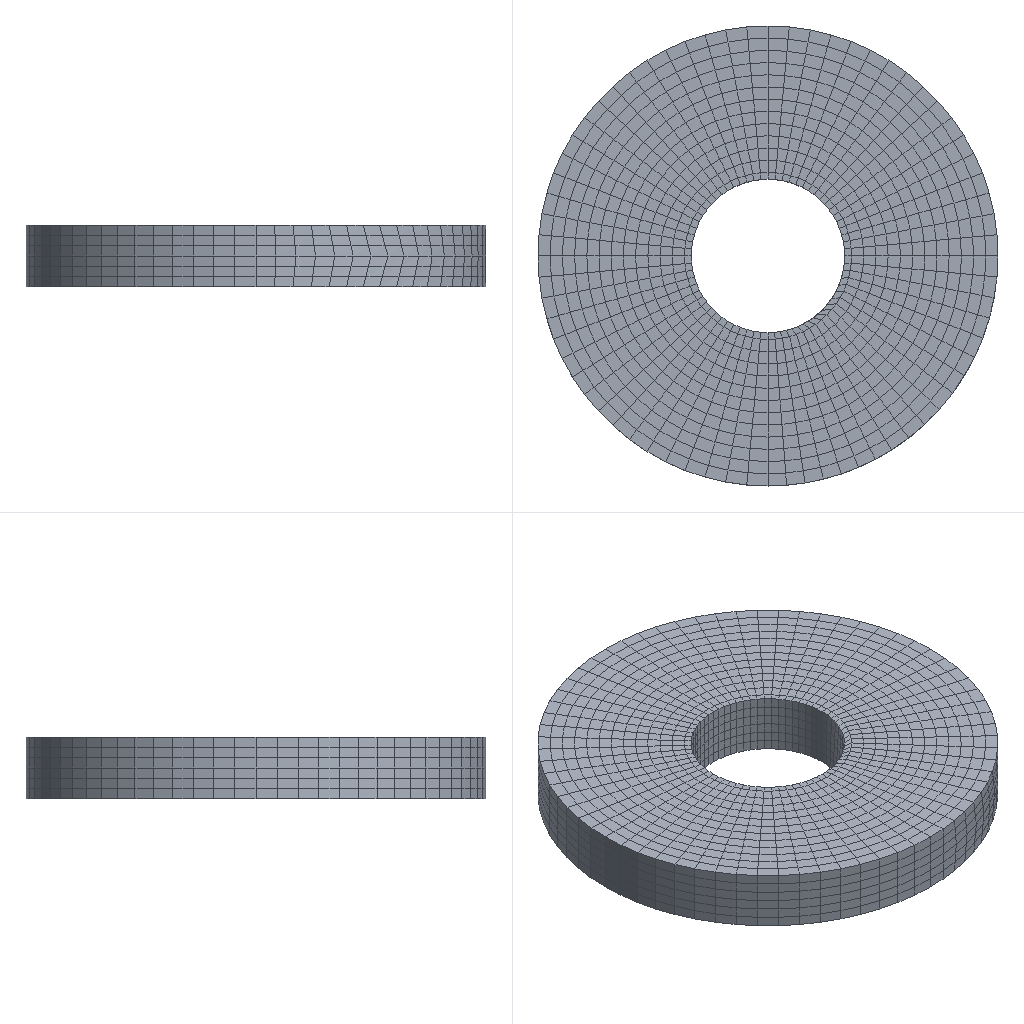Simulation study | abaqus
Set-up summary:
category,name,step,type,value,unit,region
solver,abaqus
solver,version,,,Abaqus/Standard 2020
units,not stated in the deck,,not stated
analysis,deck,,transient,transient
load_step,Step-1,Step-1,transient
load_step,requested,,,1
mesh,nodes,,,8353
mesh,elements,,,6735
element_type,C3D8,,solid,5382
element_type,R3D3,,rigid,14
element_type,R3D4,,rigid,1270
element_type,COH3D8,,cohesive,69
load,load commands in deck,,count,1
bc,support commands in deck,,count,1
material,MATERIAL-1,,in results
material,MATERIAL-1-COPY,,in results
check,setup vs results,,match,"per instance, exact: element labels, types and connectivity; labels of the nodes the elements use; coordinates of those nodes at SINGLE_PRECISION in 2 of 2 instance(s)"
Abaqus input file, long lists of numbers shortened:
*Heading
** Job name: Job-2 Model name: Model-1-Copy
** Generated by: Abaqus/CAE 2020
*Preprint, echo=NO, model=NO, history=NO, contact=NO
**
** PARTS
**
*Part, name=Part-1
*Node
      1,   1.118,  -2.236,           4.
      2,   1.118,  -2.236,           0.
** (1277 more lines like these left out)
*Element, type=R3D4
  1,   1,   3, 105, 156
  2,   3,   4, 106, 105
** (1268 more lines like these left out)
*Element, type=R3D3
677,  963,  757,  736
678,  987,  863,  818
** (12 more lines like these left out)
*Node
   1280,           0., -1.5308085e-16,           4.
*Nset, nset=Part-1-RefPt_, internal
1280,
*Elset, elset=Part-1, generate
    1,  1284,     1
*End Part
**
*Part, name=Part-2
*Node
      1,   2.723,           0.,           1.
      2,          2.5,           0.,           1.
** (7071 more lines like these left out)
*Element, type=C3D8
 1,  108,  111,  834,  802,    1, 6763, 6764,   72
 2,  802,  834,  835,  803,   72, 6764, 6765,   71
** (5380 more lines like these left out)
*Element, type=COH3D8
5383,   72,   41,    2,    1,   72, 6764, 6763,    1
5384,   71,   42,   41,   72,   71, 6765, 6764,   72
** (67 more lines like these left out)
*Nset, nset=Set-3, generate
    1,  6831,     1
*Elset, elset=Set-3, generate
    1,  5382,     1
*Nset, nset=Set-11
    1,    4,    7,    8,    9,   13,   14,   17,   18,   19,   20,   21,   22,   23,   24,   25
   26,   27,   30,   31,   34,   36,   37,   38,   39,   40,   57,   58,   59,   60,   61,   62
** (391 more lines like these left out)
*Elset, elset=Set-11
  157,  158,  159,  160,  161,  162,  163,  164,  165,  166,  167,  168,  169,  170,  171,  172
  173,  174,  175,  176,  177,  178,  179,  180,  181,  182,  183,  184,  185,  186,  187,  188
** (309 more lines like these left out)
*Nset, nset=Set-12, generate
    1,  6831,     1
*Elset, elset=Set-12, generate
    1,  5382,     1
*Elset, elset=CohesiveSeam-1-Elements, generate
 5383,  5451,     1
*Nset, nset=CohesiveSeam-1-TopNodes
    1,    4,    9,   14,   57,   58,   59,   60,   61,   62,   63,   64,   65,   66,   67,   68
   69,   70,   71,   72,  130,  131,  132,  133,  134,  135,  136,  137,  138,  139,  140,  141
** (7 more lines like these left out)
*Nset, nset=CohesiveSeam-1-BottomNodes
   1,   2,   3,   4,   9,  10,  14,  15,  41,  42,  43,  44,  45,  46,  47,  48
  49,  50,  51,  52,  53,  54,  55,  56,  57,  58,  59,  60,  61,  62,  63,  64
** (7 more lines like these left out)
*Nset, nset=CohesiveSeam-1-MidNodes
   1,   4,   9,  14,  57,  58,  59,  60,  61,  62,  63,  64,  65,  66,  67,  68
  69,  70,  71,  72, 130, 131, 132, 133, 134, 135, 136, 137, 138, 139, 140, 141
** (3 more lines like these left out)
*Elset, elset=__PickedSurf25_S1, internal, generate
 5383,  5451,     1
*Surface, type=ELEMENT, name=_PickedSurf25, internal
__PickedSurf25_S1, S1
*Elset, elset=_CohesiveSeam-1-TopSurf_S2, internal, generate
 5383,  5451,     1
*Surface, type=ELEMENT, name=CohesiveSeam-1-TopSurf
_CohesiveSeam-1-TopSurf_S2, S2
*Elset, elset=_CohesiveSeam-1-BottomSurf_S1, internal, generate
 5383,  5451,     1
*Surface, type=ELEMENT, name=CohesiveSeam-1-BottomSurf
_CohesiveSeam-1-BottomSurf_S1, S1
** Section: Section-1
*Solid Section, elset=Set-12, material=Material-1
,
** Section: Section-coh
*Cohesive Section, elset=CohesiveSeam-1-Elements, controls=EC-1, material=Material-1-Copy, response=TRACTION SEPARATION
,
*End Part
**
**
** ASSEMBLY
**
*Assembly, name=Assembly
**
*Instance, name=Part-1-1, part=Part-1
*End Instance
**
*Instance, name=Part-2-1, part=Part-2
          0.,           0.,           1.
*End Instance
**
*Nset, nset=Set-1, instance=Part-1-1
    1,    2,    3,    4,    5,    6,    7,    8,    9,   10,   11,   12,   13,   14,   15,   16
   17,   18,   19,   20,   21,   22,   23,   24,   25,   26,   27,   28,   29,   30,   31,   32
** (39 more lines like these left out)
*Elset, elset=Set-1, instance=Part-1-1, generate
  677,  1284,     1
*Nset, nset=Set-2, instance=Part-1-1
 1280,
*Elset, elset=_Surf-7_S5, internal, instance=Part-2-1
  967,  968,  969,  970,  971,  972,  973,  974,  975,  976,  977,  978,  979,  980,  981,  982
  983,  984, 1183, 1184, 1185, 1186, 1187, 1188, 1189, 1190, 1191, 1192, 1193, 1194, 1195, 1196
** (15 more lines like these left out)
*Elset, elset=_Surf-7_S3, internal, instance=Part-2-1
  157,  158,  159,  160,  161,  162,  163,  164,  165,  166,  167,  168,  169,  170,  171,  172
  173,  361,  362,  363,  364,  365,  366,  367,  368,  369,  370,  371,  372,  373,  374,  375
** (5 more lines like these left out)
*Elset, elset=_Surf-7_S6, internal, instance=Part-2-1, generate
 4159,  4759,    12
*Surface, type=ELEMENT, name=Surf-7
_Surf-7_S5, S5
_Surf-7_S3, S3
_Surf-7_S6, S6
*Elset, elset=_m_Surf-1_SPOS, internal, instance=Part-1-1, generate
   1,  676,    1
*Surface, type=ELEMENT, name=m_Surf-1
_m_Surf-1_SPOS, SPOS
*Elset, elset=_m_Surf-4_SPOS, internal, instance=Part-1-1, generate
   1,  676,    1
*Surface, type=ELEMENT, name=m_Surf-4
_m_Surf-4_SPOS, SPOS
*Elset, elset=_s_Surf-8_S4, internal, instance=Part-2-1
    1,    2,    3,    4,    5,    6,    7,    8,    9,   10,   11,   12,   13,   14,   15,   16
   17,   18,   19,   20,   21,   22,   23,   24,   25,   26,   27,   28,   29,   30,   31,   32
** (12 more lines like these left out)
*Elset, elset=_s_Surf-8_S5, internal, instance=Part-2-1
  106,  107,  108,  109,  110,  111,  112,  113,  114,  115,  116,  117,  118,  119,  120,  121
  122,  123,  124,  125,  126,  127,  128,  129,  130,  131,  132,  133,  134,  135,  136,  137
** (11 more lines like these left out)
*Surface, type=ELEMENT, name=s_Surf-8
_s_Surf-8_S4, S4
_s_Surf-8_S5, S5
*Rigid Body, ref node=Part-1-1.Part-1-RefPt_, elset=Part-1-1.Part-1
*End Assembly
**
** ELEMENT CONTROLS
**
*Section Controls, name=EC-1, ELEMENT DELETION=YES
1., 1., 1.
*Amplitude, name=Amp-1
             0.,              0.,              1.,              1.
**
** MATERIALS
**
*Material, name=Material-1
*Density
 1e-09,
*Elastic
75800., 0.24
*Material, name=Material-1-Copy
*Damage Initiation, criterion=QUADS
5.,1.,1.
*Damage Evolution, type=DISPLACEMENT
 1e-06,
*Density
 1e-09,
*Elastic, type=TRACTION
70000.,56000.,56000.
**
** INTERACTION PROPERTIES
**
*Surface Interaction, name=IntProp-1
1.,
*Friction, slip tolerance=0.005
 0.2,
*Surface Behavior, pressure-overclosure=HARD
*Surface Interaction, name=IntProp-2
1.,
** ----------------------------------------------------------------
**
** STEP: Step-1
**
*Step, name=Step-1, nlgeom=YES, inc=1000
*Dynamic
0.001,1.,1e-05
**
** BOUNDARY CONDITIONS
**
** Name: BC-1 Type: 对称/反对称/完全固定
*Boundary
Set-2, ENCASTRE
**
** LOADS
**
** Name: Load-1   Type: Pressure
*Dsload, amplitude=Amp-1
Surf-7, P, 50.
**
** OUTPUT REQUESTS
**
*Restart, write, number interval=1, time marks=NO
**
** FIELD OUTPUT: F-Output-1
**
*Output, field, number interval=20, time marks=NO
*Node Output
CF, RF, U, V
*Element Output, directions=YES
DMICRT, E, EACTIVE, LE, MISES, MISESMAX, PE, PEEQ, PEMAG, S, SDEG, STATUS
*Contact Output
CSDMG,
**
** HISTORY OUTPUT: H-Output-1
**
*Output, history, variable=PRESELECT, frequency=1
*End Step
Results summary:
result,step,,partial,increments=79 time=0.1299/1.0
result,analysis,,,transient
result,last_loadstep,,,1
result,primary field,,,U
result,reaction total,,FX,0.0,model units
result,reaction total,,FY,0.0,model units
result,reaction total,,FZ,0.0,model units